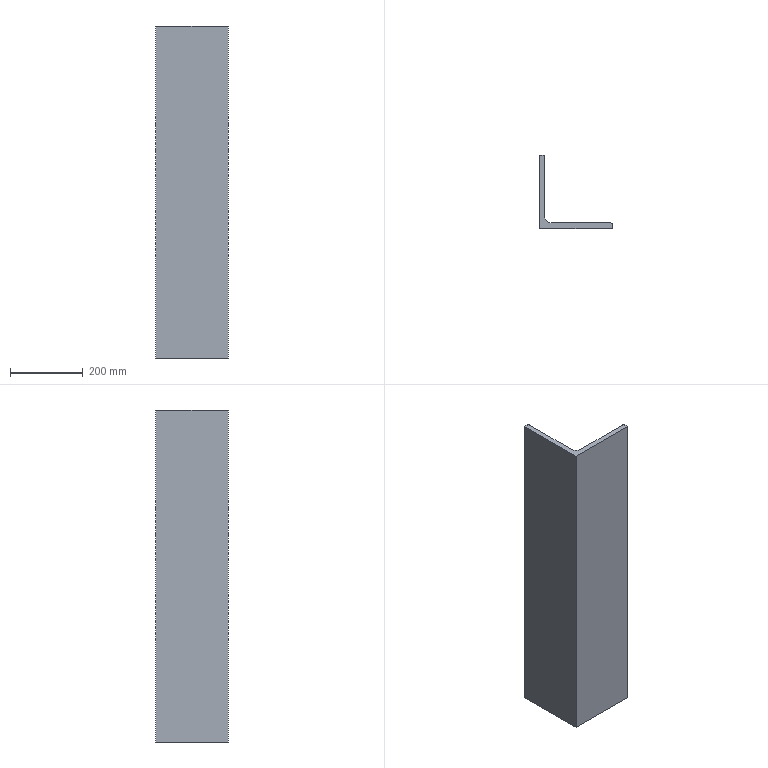Part | SolidWorks | features Extrusion 1 | 1 solid | 11 faces | box 200 x 200 x 914.4 mm | volume 4996450 mm3 | plane 8 | cylinder 3 | commonest cylinder face diameters 9.333 x2 36 x1
STEP:
#1=CARTESIAN_POINT('',(9.333,200.,-457.2));
#2=VERTEX_POINT('',#1);
#3=CARTESIAN_POINT('',(0.,200.,-457.2));
#4=VERTEX_POINT('',#3);
#5=CARTESIAN_POINT('',(0.,200.,-457.2));
#6=DIRECTION('',(-1.,0.,0.));
#7=VECTOR('',#6,1000.);
#8=LINE('',#5,#7);
#9=EDGE_CURVE('',#2,#4,#8,.T.);
#10=ORIENTED_EDGE('',*,*,#9,.T.);
#11=CARTESIAN_POINT('',(0.,200.,457.2));
#12=VERTEX_POINT('',#11);
#13=CARTESIAN_POINT('',(0.,200.,457.2));
#14=DIRECTION('',(0.,0.,-1.));
#15=VECTOR('',#14,1000.);
#16=LINE('',#13,#15);
#17=EDGE_CURVE('',#12,#4,#16,.T.);
#18=ORIENTED_EDGE('',*,*,#17,.F.);
#19=CARTESIAN_POINT('',(9.333,200.,457.2));
#20=VERTEX_POINT('',#19);
#21=CARTESIAN_POINT('',(0.,200.,457.2));
#22=DIRECTION('',(-1.,0.,0.));
#23=VECTOR('',#22,1000.);
#24=LINE('',#21,#23);
#25=EDGE_CURVE('',#20,#12,#24,.T.);
#26=ORIENTED_EDGE('',*,*,#25,.F.);
#27=CARTESIAN_POINT('',(9.333,200.,457.2));
#28=DIRECTION('',(0.,0.,-1.));
#29=VECTOR('',#28,1000.);
#30=LINE('',#27,#29);
#31=EDGE_CURVE('',#20,#2,#30,.T.);
#32=ORIENTED_EDGE('',*,*,#31,.T.);
#33=EDGE_LOOP('',(#10,#18,#26,#32));
#34=FACE_OUTER_BOUND('',#33,.T.);
#35=CARTESIAN_POINT('',(0.,200.,457.2));
#36=DIRECTION('',(0.,-1.,0.));
#37=DIRECTION('',(0.,0.,-1.));
#38=AXIS2_PLACEMENT_3D('',#35,#36,#37);
#39=PLANE('',#38);
#40=ADVANCED_FACE('',(#34),#39,.F.);
#41=CARTESIAN_POINT('',(0.,0.,-457.2));
#42=VERTEX_POINT('',#41);
#43=CARTESIAN_POINT('',(0.,200.,-457.2));
#44=DIRECTION('',(0.,-1.,0.));
#45=VECTOR('',#44,1000.);
#46=LINE('',#43,#45);
#47=EDGE_CURVE('',#4,#42,#46,.T.);
#48=ORIENTED_EDGE('',*,*,#47,.T.);
#49=CARTESIAN_POINT('',(0.,0.,457.2));
#50=VERTEX_POINT('',#49);
#51=CARTESIAN_POINT('',(0.,0.,457.2));
#52=DIRECTION('',(0.,0.,-1.));
#53=VECTOR('',#52,1000.);
#54=LINE('',#51,#53);
#55=EDGE_CURVE('',#50,#42,#54,.T.);
#56=ORIENTED_EDGE('',*,*,#55,.F.);
#57=CARTESIAN_POINT('',(0.,200.,457.2));
#58=DIRECTION('',(0.,-1.,0.));
#59=VECTOR('',#58,1000.);
#60=LINE('',#57,#59);
#61=EDGE_CURVE('',#12,#50,#60,.T.);
#62=ORIENTED_EDGE('',*,*,#61,.F.);
#63=ORIENTED_EDGE('',*,*,#17,.T.);
#64=EDGE_LOOP('',(#48,#56,#62,#63));
#65=FACE_OUTER_BOUND('',#64,.T.);
#66=CARTESIAN_POINT('',(0.,200.,457.2));
#67=DIRECTION('',(1.,0.,0.));
#68=DIRECTION('',(0.,1.,0.));
#69=AXIS2_PLACEMENT_3D('',#66,#67,#68);
#70=PLANE('',#69);
#71=ADVANCED_FACE('',(#65),#70,.F.);
#72=CARTESIAN_POINT('',(200.,0.,-457.2));
#73=VERTEX_POINT('',#72);
#74=CARTESIAN_POINT('',(0.,0.,-457.2));
#75=DIRECTION('',(1.,0.,0.));
#76=VECTOR('',#75,1000.);
#77=LINE('',#74,#76);
#78=EDGE_CURVE('',#42,#73,#77,.T.);
#79=ORIENTED_EDGE('',*,*,#78,.T.);
#80=CARTESIAN_POINT('',(200.,0.,457.2));
#81=VERTEX_POINT('',#80);
#82=CARTESIAN_POINT('',(200.,0.,457.2));
#83=DIRECTION('',(0.,0.,-1.));
#84=VECTOR('',#83,1000.);
#85=LINE('',#82,#84);
#86=EDGE_CURVE('',#81,#73,#85,.T.);
#87=ORIENTED_EDGE('',*,*,#86,.F.);
#88=CARTESIAN_POINT('',(0.,0.,457.2));
#89=DIRECTION('',(1.,0.,0.));
#90=VECTOR('',#89,1000.);
#91=LINE('',#88,#90);
#92=EDGE_CURVE('',#50,#81,#91,.T.);
#93=ORIENTED_EDGE('',*,*,#92,.F.);
#94=ORIENTED_EDGE('',*,*,#55,.T.);
#95=EDGE_LOOP('',(#79,#87,#93,#94));
#96=FACE_OUTER_BOUND('',#95,.T.);
#97=CARTESIAN_POINT('',(0.,0.,457.2));
#98=DIRECTION('',(0.,1.,0.));
#99=DIRECTION('',(0.,0.,1.));
#100=AXIS2_PLACEMENT_3D('',#97,#98,#99);
#101=PLANE('',#100);
#102=ADVANCED_FACE('',(#96),#101,.F.);
#103=CARTESIAN_POINT('',(200.,9.333,-457.2));
#104=VERTEX_POINT('',#103);
#105=CARTESIAN_POINT('',(200.,0.,-457.2));
#106=DIRECTION('',(0.,1.,0.));
#107=VECTOR('',#106,1000.);
#108=LINE('',#105,#107);
#109=EDGE_CURVE('',#73,#104,#108,.T.);
#110=ORIENTED_EDGE('',*,*,#109,.T.);
#111=CARTESIAN_POINT('',(200.,9.333,457.2));
#112=VERTEX_POINT('',#111);
#113=CARTESIAN_POINT('',(200.,9.333,457.2));
#114=DIRECTION('',(0.,0.,-1.));
#115=VECTOR('',#114,1000.);
#116=LINE('',#113,#115);
#117=EDGE_CURVE('',#112,#104,#116,.T.);
#118=ORIENTED_EDGE('',*,*,#117,.F.);
#119=CARTESIAN_POINT('',(200.,0.,457.2));
#120=DIRECTION('',(0.,1.,0.));
#121=VECTOR('',#120,1000.);
#122=LINE('',#119,#121);
#123=EDGE_CURVE('',#81,#112,#122,.T.);
#124=ORIENTED_EDGE('',*,*,#123,.F.);
#125=ORIENTED_EDGE('',*,*,#86,.T.);
#126=EDGE_LOOP('',(#110,#118,#124,#125));
#127=FACE_OUTER_BOUND('',#126,.T.);
#128=CARTESIAN_POINT('',(200.,0.,457.2));
#129=DIRECTION('',(-1.,0.,0.));
#130=DIRECTION('',(0.,0.,1.));
#131=AXIS2_PLACEMENT_3D('',#128,#129,#130);
#132=PLANE('',#131);
#133=ADVANCED_FACE('',(#127),#132,.F.);
#134=CARTESIAN_POINT('',(195.333,14.,-457.2));
#135=VERTEX_POINT('',#134);
#136=CARTESIAN_POINT('',(195.333,9.333,-457.2));
#137=DIRECTION('',(0.,0.,1.));
#138=DIRECTION('',(1.,0.,0.));
#139=AXIS2_PLACEMENT_3D('',#136,#137,#138);
#140=CIRCLE('',#139,4.667);
#141=EDGE_CURVE('',#104,#135,#140,.T.);
#142=ORIENTED_EDGE('',*,*,#141,.T.);
#143=CARTESIAN_POINT('',(195.333,14.,457.2));
#144=VERTEX_POINT('',#143);
#145=CARTESIAN_POINT('',(195.333,14.,457.2));
#146=DIRECTION('',(0.,0.,-1.));
#147=VECTOR('',#146,1000.);
#148=LINE('',#145,#147);
#149=EDGE_CURVE('',#144,#135,#148,.T.);
#150=ORIENTED_EDGE('',*,*,#149,.F.);
#151=CARTESIAN_POINT('',(195.333,9.333,457.2));
#152=DIRECTION('',(0.,0.,1.));
#153=DIRECTION('',(1.,0.,0.));
#154=AXIS2_PLACEMENT_3D('',#151,#152,#153);
#155=CIRCLE('',#154,4.667);
#156=EDGE_CURVE('',#112,#144,#155,.T.);
#157=ORIENTED_EDGE('',*,*,#156,.F.);
#158=ORIENTED_EDGE('',*,*,#117,.T.);
#159=EDGE_LOOP('',(#142,#150,#157,#158));
#160=FACE_OUTER_BOUND('',#159,.T.);
#161=CARTESIAN_POINT('',(195.333,9.333,457.2));
#162=DIRECTION('',(0.,0.,-1.));
#163=DIRECTION('',(-1.,0.,0.));
#164=AXIS2_PLACEMENT_3D('',#161,#162,#163);
#165=CYLINDRICAL_SURFACE('',#164,4.667);
#166=ADVANCED_FACE('',(#160),#165,.T.);
#167=CARTESIAN_POINT('',(32.,14.,-457.2));
#168=VERTEX_POINT('',#167);
#169=CARTESIAN_POINT('',(32.,14.,-457.2));
#170=DIRECTION('',(-1.,0.,0.));
#171=VECTOR('',#170,1000.);
#172=LINE('',#169,#171);
#173=EDGE_CURVE('',#135,#168,#172,.T.);
#174=ORIENTED_EDGE('',*,*,#173,.T.);
#175=CARTESIAN_POINT('',(32.,14.,457.2));
#176=VERTEX_POINT('',#175);
#177=CARTESIAN_POINT('',(32.,14.,457.2));
#178=DIRECTION('',(0.,0.,-1.));
#179=VECTOR('',#178,1000.);
#180=LINE('',#177,#179);
#181=EDGE_CURVE('',#176,#168,#180,.T.);
#182=ORIENTED_EDGE('',*,*,#181,.F.);
#183=CARTESIAN_POINT('',(32.,14.,457.2));
#184=DIRECTION('',(-1.,0.,0.));
#185=VECTOR('',#184,1000.);
#186=LINE('',#183,#185);
#187=EDGE_CURVE('',#144,#176,#186,.T.);
#188=ORIENTED_EDGE('',*,*,#187,.F.);
#189=ORIENTED_EDGE('',*,*,#149,.T.);
#190=EDGE_LOOP('',(#174,#182,#188,#189));
#191=FACE_OUTER_BOUND('',#190,.T.);
#192=CARTESIAN_POINT('',(32.,14.,457.2));
#193=DIRECTION('',(0.,-1.,0.));
#194=DIRECTION('',(0.,0.,-1.));
#195=AXIS2_PLACEMENT_3D('',#192,#193,#194);
#196=PLANE('',#195);
#197=ADVANCED_FACE('',(#191),#196,.F.);
#198=CARTESIAN_POINT('',(14.,32.,-457.2));
#199=VERTEX_POINT('',#198);
#200=CARTESIAN_POINT('',(32.,32.,-457.2));
#201=DIRECTION('',(0.,0.,-1.));
#202=DIRECTION('',(1.,0.,0.));
#203=AXIS2_PLACEMENT_3D('',#200,#201,#202);
#204=CIRCLE('',#203,18.);
#205=EDGE_CURVE('',#168,#199,#204,.T.);
#206=ORIENTED_EDGE('',*,*,#205,.T.);
#207=CARTESIAN_POINT('',(14.,32.,457.2));
#208=VERTEX_POINT('',#207);
#209=CARTESIAN_POINT('',(14.,32.,457.2));
#210=DIRECTION('',(0.,0.,-1.));
#211=VECTOR('',#210,1000.);
#212=LINE('',#209,#211);
#213=EDGE_CURVE('',#208,#199,#212,.T.);
#214=ORIENTED_EDGE('',*,*,#213,.F.);
#215=CARTESIAN_POINT('',(32.,32.,457.2));
#216=DIRECTION('',(0.,0.,-1.));
#217=DIRECTION('',(1.,0.,0.));
#218=AXIS2_PLACEMENT_3D('',#215,#216,#217);
#219=CIRCLE('',#218,18.);
#220=EDGE_CURVE('',#176,#208,#219,.T.);
#221=ORIENTED_EDGE('',*,*,#220,.F.);
#222=ORIENTED_EDGE('',*,*,#181,.T.);
#223=EDGE_LOOP('',(#206,#214,#221,#222));
#224=FACE_OUTER_BOUND('',#223,.T.);
#225=CARTESIAN_POINT('',(32.,32.,457.2));
#226=DIRECTION('',(0.,0.,-1.));
#227=DIRECTION('',(-1.,0.,0.));
#228=AXIS2_PLACEMENT_3D('',#225,#226,#227);
#229=CYLINDRICAL_SURFACE('',#228,18.);
#230=ADVANCED_FACE('',(#224),#229,.F.);
#231=CARTESIAN_POINT('',(14.,195.333,-457.2));
#232=VERTEX_POINT('',#231);
#233=CARTESIAN_POINT('',(14.,195.333,-457.2));
#234=DIRECTION('',(0.,1.,0.));
#235=VECTOR('',#234,1000.);
#236=LINE('',#233,#235);
#237=EDGE_CURVE('',#199,#232,#236,.T.);
#238=ORIENTED_EDGE('',*,*,#237,.T.);
#239=CARTESIAN_POINT('',(14.,195.333,457.2));
#240=VERTEX_POINT('',#239);
#241=CARTESIAN_POINT('',(14.,195.333,457.2));
#242=DIRECTION('',(0.,0.,-1.));
#243=VECTOR('',#242,1000.);
#244=LINE('',#241,#243);
#245=EDGE_CURVE('',#240,#232,#244,.T.);
#246=ORIENTED_EDGE('',*,*,#245,.F.);
#247=CARTESIAN_POINT('',(14.,195.333,457.2));
#248=DIRECTION('',(0.,1.,0.));
#249=VECTOR('',#248,1000.);
#250=LINE('',#247,#249);
#251=EDGE_CURVE('',#208,#240,#250,.T.);
#252=ORIENTED_EDGE('',*,*,#251,.F.);
#253=ORIENTED_EDGE('',*,*,#213,.T.);
#254=EDGE_LOOP('',(#238,#246,#252,#253));
#255=FACE_OUTER_BOUND('',#254,.T.);
#256=CARTESIAN_POINT('',(14.,195.333,457.2));
#257=DIRECTION('',(-1.,0.,0.));
#258=DIRECTION('',(0.,-1.,0.));
#259=AXIS2_PLACEMENT_3D('',#256,#257,#258);
#260=PLANE('',#259);
#261=ADVANCED_FACE('',(#255),#260,.F.);
#262=CARTESIAN_POINT('',(9.333,195.333,-457.2));
#263=DIRECTION('',(0.,0.,1.));
#264=DIRECTION('',(-1.,0.,0.));
#265=AXIS2_PLACEMENT_3D('',#262,#263,#264);
#266=CIRCLE('',#265,4.667);
#267=EDGE_CURVE('',#232,#2,#266,.T.);
#268=ORIENTED_EDGE('',*,*,#267,.T.);
#269=ORIENTED_EDGE('',*,*,#31,.F.);
#270=CARTESIAN_POINT('',(9.333,195.333,457.2));
#271=DIRECTION('',(0.,0.,1.));
#272=DIRECTION('',(-1.,0.,0.));
#273=AXIS2_PLACEMENT_3D('',#270,#271,#272);
#274=CIRCLE('',#273,4.667);
#275=EDGE_CURVE('',#240,#20,#274,.T.);
#276=ORIENTED_EDGE('',*,*,#275,.F.);
#277=ORIENTED_EDGE('',*,*,#245,.T.);
#278=EDGE_LOOP('',(#268,#269,#276,#277));
#279=FACE_OUTER_BOUND('',#278,.T.);
#280=CARTESIAN_POINT('',(9.333,195.333,457.2));
#281=DIRECTION('',(0.,0.,-1.));
#282=DIRECTION('',(-1.,0.,0.));
#283=AXIS2_PLACEMENT_3D('',#280,#281,#282);
#284=CYLINDRICAL_SURFACE('',#283,4.667);
#285=ADVANCED_FACE('',(#279),#284,.T.);
#286=ORIENTED_EDGE('',*,*,#25,.T.);
#287=ORIENTED_EDGE('',*,*,#61,.T.);
#288=ORIENTED_EDGE('',*,*,#92,.T.);
#289=ORIENTED_EDGE('',*,*,#123,.T.);
#290=ORIENTED_EDGE('',*,*,#156,.T.);
#291=ORIENTED_EDGE('',*,*,#187,.T.);
#292=ORIENTED_EDGE('',*,*,#220,.T.);
#293=ORIENTED_EDGE('',*,*,#251,.T.);
#294=ORIENTED_EDGE('',*,*,#275,.T.);
#295=EDGE_LOOP('',(#286,#287,#288,#289,#290,#291,#292,#293,#294));
#296=FACE_OUTER_BOUND('',#295,.T.);
#297=CARTESIAN_POINT('',(9.333,195.333,457.2));
#298=DIRECTION('',(0.,0.,-1.));
#299=DIRECTION('',(-1.,0.,0.));
#300=AXIS2_PLACEMENT_3D('',#297,#298,#299);
#301=PLANE('',#300);
#302=ADVANCED_FACE('',(#296),#301,.F.);
#303=ORIENTED_EDGE('',*,*,#9,.F.);
#304=ORIENTED_EDGE('',*,*,#267,.F.);
#305=ORIENTED_EDGE('',*,*,#237,.F.);
#306=ORIENTED_EDGE('',*,*,#205,.F.);
#307=ORIENTED_EDGE('',*,*,#173,.F.);
#308=ORIENTED_EDGE('',*,*,#141,.F.);
#309=ORIENTED_EDGE('',*,*,#109,.F.);
#310=ORIENTED_EDGE('',*,*,#78,.F.);
#311=ORIENTED_EDGE('',*,*,#47,.F.);
#312=EDGE_LOOP('',(#303,#304,#305,#306,#307,#308,#309,#310,#311));
#313=FACE_OUTER_BOUND('',#312,.T.);
#314=CARTESIAN_POINT('',(9.333,195.333,-457.2));
#315=DIRECTION('',(0.,0.,-1.));
#316=DIRECTION('',(-1.,0.,0.));
#317=AXIS2_PLACEMENT_3D('',#314,#315,#316);
#318=PLANE('',#317);
#319=ADVANCED_FACE('',(#313),#318,.T.);
#320=CLOSED_SHELL('',(#40,#71,#102,#133,#166,#197,#230,#261,#285,#302,#319));
#321=MANIFOLD_SOLID_BREP('',#320);
#322=CARTESIAN_POINT('',(0.,0.,0.));
#323=DIRECTION('',(0.,0.,1.));
#324=DIRECTION('',(1.,0.,0.));
#325=AXIS2_PLACEMENT_3D('',#322,#323,#324);
#326=(LENGTH_UNIT()NAMED_UNIT(*)SI_UNIT(.MILLI.,.METRE.));
#327=UNCERTAINTY_MEASURE_WITH_UNIT(LENGTH_MEASURE(0.00001),#326,'','');
#328=(NAMED_UNIT(*)PLANE_ANGLE_UNIT()SI_UNIT($,.RADIAN.));
#329=(NAMED_UNIT(*)SI_UNIT($,.STERADIAN.)SOLID_ANGLE_UNIT());
#330=(GEOMETRIC_REPRESENTATION_CONTEXT(3)GLOBAL_UNCERTAINTY_ASSIGNED_CONTEXT((#327))GLOBAL_UNIT_ASSIGNED_CONTEXT((#326,#328,#329))REPRESENTATION_CONTEXT('',''));
#331=ADVANCED_BREP_SHAPE_REPRESENTATION('',(#321,#325),#330);